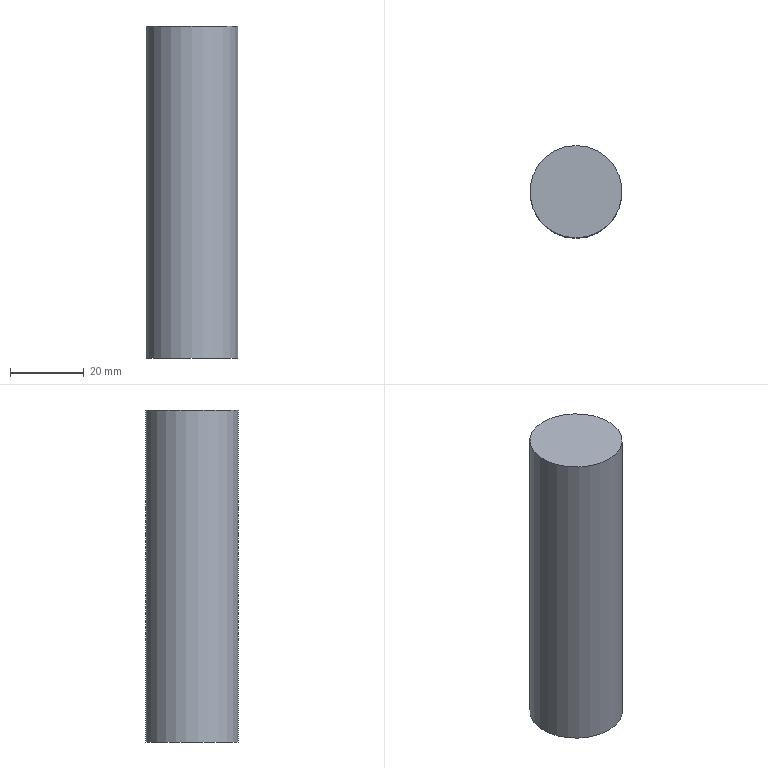Part | NX | features solid 2 | 1 solid | 3 faces | box 25 x 25 x 90 mm | volume 44179 mm3 | plane 2 | cylinder 1 | commonest cylinder face diameters 25 x1
STEP:
#1=CARTESIAN_POINT('',(285.,17.5,195.));
#2=VERTEX_POINT('',#1);
#3=CARTESIAN_POINT('',(285.,5.,195.));
#4=DIRECTION('',(0.,0.,-1.));
#5=DIRECTION('',(0.,1.,0.));
#6=AXIS2_PLACEMENT_3D('',#3,#4,#5);
#7=CIRCLE('',#6,12.5);
#8=EDGE_CURVE('',#2,#2,#7,.T.);
#9=ORIENTED_EDGE('',*,*,#8,.F.);
#10=EDGE_LOOP('',(#9));
#11=FACE_BOUND('',#10,.T.);
#12=CARTESIAN_POINT('',(285.,17.5,285.));
#13=VERTEX_POINT('',#12);
#14=CARTESIAN_POINT('',(285.,5.,285.));
#15=DIRECTION('',(0.,0.,-1.));
#16=DIRECTION('',(0.,1.,0.));
#17=AXIS2_PLACEMENT_3D('',#14,#15,#16);
#18=CIRCLE('',#17,12.5);
#19=EDGE_CURVE('',#13,#13,#18,.T.);
#20=ORIENTED_EDGE('',*,*,#19,.T.);
#21=EDGE_LOOP('',(#20));
#22=FACE_BOUND('',#21,.T.);
#23=CARTESIAN_POINT('',(285.,5.,291.25));
#24=DIRECTION('',(0.,0.,1.));
#25=DIRECTION('',(0.,-1.,0.));
#26=AXIS2_PLACEMENT_3D('',#23,#24,#25);
#27=CYLINDRICAL_SURFACE('',#26,12.5);
#28=ADVANCED_FACE('',(#11,#22),#27,.T.);
#29=ORIENTED_EDGE('',*,*,#8,.T.);
#30=EDGE_LOOP('',(#29));
#31=FACE_BOUND('',#30,.T.);
#32=CARTESIAN_POINT('',(285.,5.,195.));
#33=DIRECTION('',(0.,0.,-1.));
#34=DIRECTION('',(0.,1.,0.));
#35=AXIS2_PLACEMENT_3D('',#32,#33,#34);
#36=PLANE('',#35);
#37=ADVANCED_FACE('',(#31),#36,.T.);
#38=ORIENTED_EDGE('',*,*,#19,.F.);
#39=EDGE_LOOP('',(#38));
#40=FACE_BOUND('',#39,.T.);
#41=CARTESIAN_POINT('',(285.,5.,285.));
#42=DIRECTION('',(0.,0.,-1.));
#43=DIRECTION('',(0.,1.,0.));
#44=AXIS2_PLACEMENT_3D('',#41,#42,#43);
#45=PLANE('',#44);
#46=ADVANCED_FACE('',(#40),#45,.F.);
#47=CLOSED_SHELL('',(#28,#37,#46));
#48=MANIFOLD_SOLID_BREP('',#47);
#49=(LENGTH_UNIT()NAMED_UNIT(*)SI_UNIT(.MILLI.,.METRE.));
#50=UNCERTAINTY_MEASURE_WITH_UNIT(LENGTH_MEASURE(0.00001),#49,'','');
#51=(NAMED_UNIT(*)PLANE_ANGLE_UNIT()SI_UNIT($,.RADIAN.));
#52=(NAMED_UNIT(*)SI_UNIT($,.STERADIAN.)SOLID_ANGLE_UNIT());
#53=(GEOMETRIC_REPRESENTATION_CONTEXT(3)GLOBAL_UNCERTAINTY_ASSIGNED_CONTEXT((#50))GLOBAL_UNIT_ASSIGNED_CONTEXT((#49,#51,#52))REPRESENTATION_CONTEXT('',''));
#54=ADVANCED_BREP_SHAPE_REPRESENTATION('',(#48),#53);